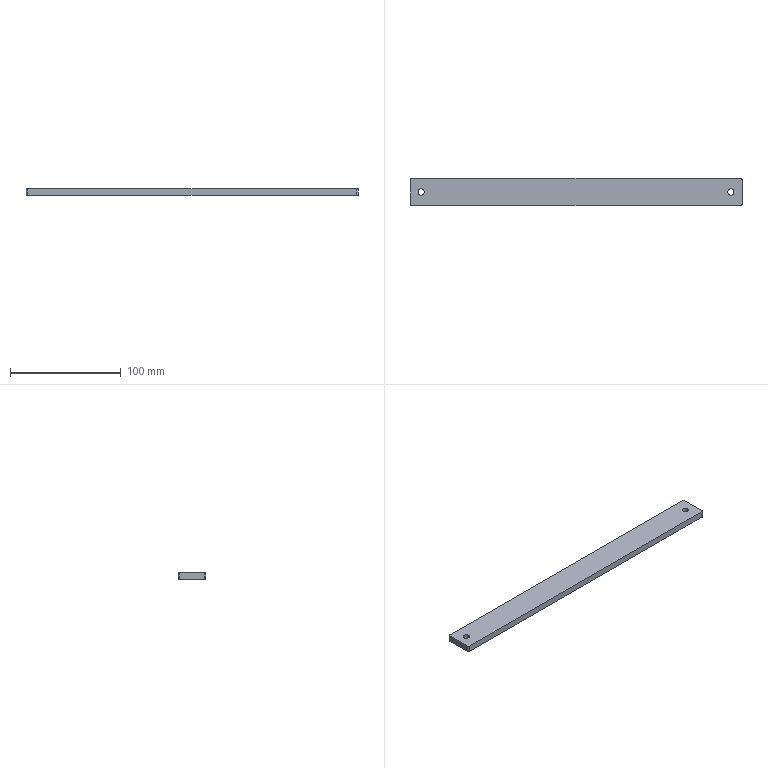Part | STEP file | PN_0032 | 1 solid | 14 faces | box 300 x 25 x 6 mm | volume 44703 mm3 | cylinder 8 | plane 6 | commonest cylinder face diameters 3 x4 5.5 x4
STEP:
#1=CARTESIAN_POINT('',(0.,0.,0.));
#2=DIRECTION('',(0.,0.,1.));
#3=DIRECTION('',(1.,0.,0.));
#4=AXIS2_PLACEMENT_3D('',#1,#2,#3);
#5=CARTESIAN_POINT('',(-137.25,0.,0.));
#6=VERTEX_POINT('',#5);
#7=CARTESIAN_POINT('',(-137.25,0.,6.));
#8=VERTEX_POINT('',#7);
#9=CARTESIAN_POINT('',(-137.25,0.,6.));
#10=DIRECTION('',(0.,0.,1.));
#11=VECTOR('',#10,1.);
#12=LINE('',#9,#11);
#13=CARTESIAN_POINT('',(-140.,0.,6.));
#14=DIRECTION('',(0.,0.,1.));
#15=DIRECTION('',(1.,0.,0.));
#16=AXIS2_PLACEMENT_3D('',#13,#14,#15);
#17=CYLINDRICAL_SURFACE('',#16,2.75);
#18=CARTESIAN_POINT('',(6.283,0.));
#19=DIRECTION('',(0.,1.));
#20=VECTOR('',#19,1.);
#21=LINE('',#18,#20);
#22=(GEOMETRIC_REPRESENTATION_CONTEXT(2)PARAMETRIC_REPRESENTATION_CONTEXT()REPRESENTATION_CONTEXT('',''));
#23=DEFINITIONAL_REPRESENTATION('',(#21),#22);
#24=PCURVE('',#17,#23);
#25=CARTESIAN_POINT('',(-140.,0.,6.));
#26=DIRECTION('',(0.,0.,1.));
#27=DIRECTION('',(1.,0.,0.));
#28=AXIS2_PLACEMENT_3D('',#25,#26,#27);
#29=CYLINDRICAL_SURFACE('',#28,2.75);
#30=CARTESIAN_POINT('',(0.,0.));
#31=DIRECTION('',(0.,1.));
#32=VECTOR('',#31,1.);
#33=LINE('',#30,#32);
#34=(GEOMETRIC_REPRESENTATION_CONTEXT(2)PARAMETRIC_REPRESENTATION_CONTEXT()REPRESENTATION_CONTEXT('',''));
#35=DEFINITIONAL_REPRESENTATION('',(#33),#34);
#36=PCURVE('',#29,#35);
#37=SURFACE_CURVE('',#12,(#24,#36),.PCURVE_S1.);
#38=EDGE_CURVE('',#6,#8,#37,.T.);
#39=ORIENTED_EDGE('',*,*,#38,.T.);
#40=CARTESIAN_POINT('',(-142.75,0.,6.));
#41=VERTEX_POINT('',#40);
#42=CARTESIAN_POINT('',(-140.,0.,6.));
#43=DIRECTION('',(0.,0.,1.));
#44=DIRECTION('',(1.,0.,0.));
#45=AXIS2_PLACEMENT_3D('',#42,#43,#44);
#46=CIRCLE('',#45,2.75);
#47=CARTESIAN_POINT('',(0.,0.));
#48=DIRECTION('',(1.,0.));
#49=VECTOR('',#48,1.);
#50=LINE('',#47,#49);
#51=(GEOMETRIC_REPRESENTATION_CONTEXT(2)PARAMETRIC_REPRESENTATION_CONTEXT()REPRESENTATION_CONTEXT('',''));
#52=DEFINITIONAL_REPRESENTATION('',(#50),#51);
#53=PCURVE('',#17,#52);
#54=CARTESIAN_POINT('',(0.,0.,6.));
#55=DIRECTION('',(0.,0.,1.));
#56=DIRECTION('',(1.,0.,0.));
#57=AXIS2_PLACEMENT_3D('',#54,#55,#56);
#58=PLANE('',#57);
#59=CARTESIAN_POINT('',(-140.,0.));
#60=DIRECTION('',(1.,0.));
#61=AXIS2_PLACEMENT_2D('',#59,#60);
#62=CIRCLE('',#61,2.75);
#63=(GEOMETRIC_REPRESENTATION_CONTEXT(2)PARAMETRIC_REPRESENTATION_CONTEXT()REPRESENTATION_CONTEXT('',''));
#64=DEFINITIONAL_REPRESENTATION('',(#62),#63);
#65=PCURVE('',#58,#64);
#66=SURFACE_CURVE('',#46,(#53,#65),.PCURVE_S1.);
#67=EDGE_CURVE('',#41,#8,#66,.T.);
#68=ORIENTED_EDGE('',*,*,#67,.F.);
#69=CARTESIAN_POINT('',(-142.75,0.,0.));
#70=VERTEX_POINT('',#69);
#71=CARTESIAN_POINT('',(-142.75,0.,6.));
#72=DIRECTION('',(0.,0.,1.));
#73=VECTOR('',#72,1.);
#74=LINE('',#71,#73);
#75=CARTESIAN_POINT('',(3.142,0.));
#76=DIRECTION('',(0.,1.));
#77=VECTOR('',#76,1.);
#78=LINE('',#75,#77);
#79=(GEOMETRIC_REPRESENTATION_CONTEXT(2)PARAMETRIC_REPRESENTATION_CONTEXT()REPRESENTATION_CONTEXT('',''));
#80=DEFINITIONAL_REPRESENTATION('',(#78),#79);
#81=PCURVE('',#17,#80);
#82=CARTESIAN_POINT('',(3.142,0.));
#83=DIRECTION('',(0.,1.));
#84=VECTOR('',#83,1.);
#85=LINE('',#82,#84);
#86=(GEOMETRIC_REPRESENTATION_CONTEXT(2)PARAMETRIC_REPRESENTATION_CONTEXT()REPRESENTATION_CONTEXT('',''));
#87=DEFINITIONAL_REPRESENTATION('',(#85),#86);
#88=PCURVE('',#29,#87);
#89=SURFACE_CURVE('',#74,(#81,#88),.PCURVE_S1.);
#90=EDGE_CURVE('',#70,#41,#89,.T.);
#91=ORIENTED_EDGE('',*,*,#90,.F.);
#92=CARTESIAN_POINT('',(-140.,0.,0.));
#93=DIRECTION('',(0.,0.,1.));
#94=DIRECTION('',(1.,0.,0.));
#95=AXIS2_PLACEMENT_3D('',#92,#93,#94);
#96=CIRCLE('',#95,2.75);
#97=CARTESIAN_POINT('',(0.,-6.));
#98=DIRECTION('',(1.,0.));
#99=VECTOR('',#98,1.);
#100=LINE('',#97,#99);
#101=(GEOMETRIC_REPRESENTATION_CONTEXT(2)PARAMETRIC_REPRESENTATION_CONTEXT()REPRESENTATION_CONTEXT('',''));
#102=DEFINITIONAL_REPRESENTATION('',(#100),#101);
#103=PCURVE('',#17,#102);
#104=CARTESIAN_POINT('',(0.,0.,0.));
#105=DIRECTION('',(0.,0.,1.));
#106=DIRECTION('',(1.,0.,0.));
#107=AXIS2_PLACEMENT_3D('',#104,#105,#106);
#108=PLANE('',#107);
#109=CARTESIAN_POINT('',(-140.,0.));
#110=DIRECTION('',(1.,0.));
#111=AXIS2_PLACEMENT_2D('',#109,#110);
#112=CIRCLE('',#111,2.75);
#113=(GEOMETRIC_REPRESENTATION_CONTEXT(2)PARAMETRIC_REPRESENTATION_CONTEXT()REPRESENTATION_CONTEXT('',''));
#114=DEFINITIONAL_REPRESENTATION('',(#112),#113);
#115=PCURVE('',#108,#114);
#116=SURFACE_CURVE('',#96,(#103,#115),.PCURVE_S1.);
#117=EDGE_CURVE('',#70,#6,#116,.T.);
#118=ORIENTED_EDGE('',*,*,#117,.T.);
#119=EDGE_LOOP('',(#39,#68,#91,#118));
#120=FACE_BOUND('',#119,.F.);
#121=ADVANCED_FACE('',(#120),#17,.F.);
#122=CARTESIAN_POINT('',(142.75,0.,0.));
#123=VERTEX_POINT('',#122);
#124=CARTESIAN_POINT('',(142.75,0.,6.));
#125=VERTEX_POINT('',#124);
#126=CARTESIAN_POINT('',(142.75,0.,6.));
#127=DIRECTION('',(0.,0.,1.));
#128=VECTOR('',#127,1.);
#129=LINE('',#126,#128);
#130=CARTESIAN_POINT('',(140.,0.,6.));
#131=DIRECTION('',(0.,0.,1.));
#132=DIRECTION('',(1.,0.,0.));
#133=AXIS2_PLACEMENT_3D('',#130,#131,#132);
#134=CYLINDRICAL_SURFACE('',#133,2.75);
#135=CARTESIAN_POINT('',(6.283,0.));
#136=DIRECTION('',(0.,1.));
#137=VECTOR('',#136,1.);
#138=LINE('',#135,#137);
#139=(GEOMETRIC_REPRESENTATION_CONTEXT(2)PARAMETRIC_REPRESENTATION_CONTEXT()REPRESENTATION_CONTEXT('',''));
#140=DEFINITIONAL_REPRESENTATION('',(#138),#139);
#141=PCURVE('',#134,#140);
#142=CARTESIAN_POINT('',(140.,0.,6.));
#143=DIRECTION('',(0.,0.,1.));
#144=DIRECTION('',(1.,0.,0.));
#145=AXIS2_PLACEMENT_3D('',#142,#143,#144);
#146=CYLINDRICAL_SURFACE('',#145,2.75);
#147=CARTESIAN_POINT('',(0.,0.));
#148=DIRECTION('',(0.,1.));
#149=VECTOR('',#148,1.);
#150=LINE('',#147,#149);
#151=(GEOMETRIC_REPRESENTATION_CONTEXT(2)PARAMETRIC_REPRESENTATION_CONTEXT()REPRESENTATION_CONTEXT('',''));
#152=DEFINITIONAL_REPRESENTATION('',(#150),#151);
#153=PCURVE('',#146,#152);
#154=SURFACE_CURVE('',#129,(#141,#153),.PCURVE_S1.);
#155=EDGE_CURVE('',#123,#125,#154,.T.);
#156=ORIENTED_EDGE('',*,*,#155,.T.);
#157=CARTESIAN_POINT('',(137.25,0.,6.));
#158=VERTEX_POINT('',#157);
#159=CARTESIAN_POINT('',(140.,0.,6.));
#160=DIRECTION('',(0.,0.,1.));
#161=DIRECTION('',(1.,0.,0.));
#162=AXIS2_PLACEMENT_3D('',#159,#160,#161);
#163=CIRCLE('',#162,2.75);
#164=CARTESIAN_POINT('',(0.,0.));
#165=DIRECTION('',(1.,0.));
#166=VECTOR('',#165,1.);
#167=LINE('',#164,#166);
#168=(GEOMETRIC_REPRESENTATION_CONTEXT(2)PARAMETRIC_REPRESENTATION_CONTEXT()REPRESENTATION_CONTEXT('',''));
#169=DEFINITIONAL_REPRESENTATION('',(#167),#168);
#170=PCURVE('',#134,#169);
#171=CARTESIAN_POINT('',(140.,0.));
#172=DIRECTION('',(1.,0.));
#173=AXIS2_PLACEMENT_2D('',#171,#172);
#174=CIRCLE('',#173,2.75);
#175=(GEOMETRIC_REPRESENTATION_CONTEXT(2)PARAMETRIC_REPRESENTATION_CONTEXT()REPRESENTATION_CONTEXT('',''));
#176=DEFINITIONAL_REPRESENTATION('',(#174),#175);
#177=PCURVE('',#58,#176);
#178=SURFACE_CURVE('',#163,(#170,#177),.PCURVE_S1.);
#179=EDGE_CURVE('',#158,#125,#178,.T.);
#180=ORIENTED_EDGE('',*,*,#179,.F.);
#181=CARTESIAN_POINT('',(137.25,0.,0.));
#182=VERTEX_POINT('',#181);
#183=CARTESIAN_POINT('',(137.25,0.,6.));
#184=DIRECTION('',(0.,0.,1.));
#185=VECTOR('',#184,1.);
#186=LINE('',#183,#185);
#187=CARTESIAN_POINT('',(3.142,0.));
#188=DIRECTION('',(0.,1.));
#189=VECTOR('',#188,1.);
#190=LINE('',#187,#189);
#191=(GEOMETRIC_REPRESENTATION_CONTEXT(2)PARAMETRIC_REPRESENTATION_CONTEXT()REPRESENTATION_CONTEXT('',''));
#192=DEFINITIONAL_REPRESENTATION('',(#190),#191);
#193=PCURVE('',#134,#192);
#194=CARTESIAN_POINT('',(3.142,0.));
#195=DIRECTION('',(0.,1.));
#196=VECTOR('',#195,1.);
#197=LINE('',#194,#196);
#198=(GEOMETRIC_REPRESENTATION_CONTEXT(2)PARAMETRIC_REPRESENTATION_CONTEXT()REPRESENTATION_CONTEXT('',''));
#199=DEFINITIONAL_REPRESENTATION('',(#197),#198);
#200=PCURVE('',#146,#199);
#201=SURFACE_CURVE('',#186,(#193,#200),.PCURVE_S1.);
#202=EDGE_CURVE('',#182,#158,#201,.T.);
#203=ORIENTED_EDGE('',*,*,#202,.F.);
#204=CARTESIAN_POINT('',(140.,0.,0.));
#205=DIRECTION('',(0.,0.,1.));
#206=DIRECTION('',(1.,0.,0.));
#207=AXIS2_PLACEMENT_3D('',#204,#205,#206);
#208=CIRCLE('',#207,2.75);
#209=CARTESIAN_POINT('',(0.,-6.));
#210=DIRECTION('',(1.,0.));
#211=VECTOR('',#210,1.);
#212=LINE('',#209,#211);
#213=(GEOMETRIC_REPRESENTATION_CONTEXT(2)PARAMETRIC_REPRESENTATION_CONTEXT()REPRESENTATION_CONTEXT('',''));
#214=DEFINITIONAL_REPRESENTATION('',(#212),#213);
#215=PCURVE('',#134,#214);
#216=CARTESIAN_POINT('',(140.,0.));
#217=DIRECTION('',(1.,0.));
#218=AXIS2_PLACEMENT_2D('',#216,#217);
#219=CIRCLE('',#218,2.75);
#220=(GEOMETRIC_REPRESENTATION_CONTEXT(2)PARAMETRIC_REPRESENTATION_CONTEXT()REPRESENTATION_CONTEXT('',''));
#221=DEFINITIONAL_REPRESENTATION('',(#219),#220);
#222=PCURVE('',#108,#221);
#223=SURFACE_CURVE('',#208,(#215,#222),.PCURVE_S1.);
#224=EDGE_CURVE('',#182,#123,#223,.T.);
#225=ORIENTED_EDGE('',*,*,#224,.T.);
#226=EDGE_LOOP('',(#156,#180,#203,#225));
#227=FACE_BOUND('',#226,.F.);
#228=ADVANCED_FACE('',(#227),#134,.F.);
#229=CARTESIAN_POINT('',(150.,-11.,6.));
#230=VERTEX_POINT('',#229);
#231=CARTESIAN_POINT('',(150.,11.,6.));
#232=VERTEX_POINT('',#231);
#233=CARTESIAN_POINT('',(150.,12.5,6.));
#234=DIRECTION('',(0.,1.,0.));
#235=VECTOR('',#234,1.);
#236=LINE('',#233,#235);
#237=CARTESIAN_POINT('',(150.,12.5,6.));
#238=DIRECTION('',(-1.,0.,0.));
#239=DIRECTION('',(0.,0.,1.));
#240=AXIS2_PLACEMENT_3D('',#237,#238,#239);
#241=PLANE('',#240);
#242=CARTESIAN_POINT('',(0.,0.));
#243=DIRECTION('',(0.,1.));
#244=VECTOR('',#243,1.);
#245=LINE('',#242,#244);
#246=(GEOMETRIC_REPRESENTATION_CONTEXT(2)PARAMETRIC_REPRESENTATION_CONTEXT()REPRESENTATION_CONTEXT('',''));
#247=DEFINITIONAL_REPRESENTATION('',(#245),#246);
#248=PCURVE('',#241,#247);
#249=CARTESIAN_POINT('',(150.,12.5));
#250=DIRECTION('',(0.,1.));
#251=VECTOR('',#250,1.);
#252=LINE('',#249,#251);
#253=(GEOMETRIC_REPRESENTATION_CONTEXT(2)PARAMETRIC_REPRESENTATION_CONTEXT()REPRESENTATION_CONTEXT('',''));
#254=DEFINITIONAL_REPRESENTATION('',(#252),#253);
#255=PCURVE('',#58,#254);
#256=SURFACE_CURVE('',#236,(#248,#255),.PCURVE_S1.);
#257=EDGE_CURVE('',#230,#232,#256,.T.);
#258=ORIENTED_EDGE('',*,*,#257,.F.);
#259=CARTESIAN_POINT('',(150.,-11.,0.));
#260=VERTEX_POINT('',#259);
#261=CARTESIAN_POINT('',(150.,-11.,6.));
#262=DIRECTION('',(0.,0.,-1.));
#263=VECTOR('',#262,1.);
#264=LINE('',#261,#263);
#265=CARTESIAN_POINT('',(0.,-23.5));
#266=DIRECTION('',(-1.,0.));
#267=VECTOR('',#266,1.);
#268=LINE('',#265,#267);
#269=(GEOMETRIC_REPRESENTATION_CONTEXT(2)PARAMETRIC_REPRESENTATION_CONTEXT()REPRESENTATION_CONTEXT('',''));
#270=DEFINITIONAL_REPRESENTATION('',(#268),#269);
#271=PCURVE('',#241,#270);
#272=CARTESIAN_POINT('',(148.5,-11.,6.));
#273=DIRECTION('',(0.,0.,-1.));
#274=DIRECTION('',(-1.,0.,0.));
#275=AXIS2_PLACEMENT_3D('',#272,#273,#274);
#276=CYLINDRICAL_SURFACE('',#275,1.5);
#277=CARTESIAN_POINT('',(3.142,0.));
#278=DIRECTION('',(0.,1.));
#279=VECTOR('',#278,1.);
#280=LINE('',#277,#279);
#281=(GEOMETRIC_REPRESENTATION_CONTEXT(2)PARAMETRIC_REPRESENTATION_CONTEXT()REPRESENTATION_CONTEXT('',''));
#282=DEFINITIONAL_REPRESENTATION('',(#280),#281);
#283=PCURVE('',#276,#282);
#284=SURFACE_CURVE('',#264,(#271,#283),.PCURVE_S1.);
#285=EDGE_CURVE('',#230,#260,#284,.T.);
#286=ORIENTED_EDGE('',*,*,#285,.T.);
#287=CARTESIAN_POINT('',(150.,11.,0.));
#288=VERTEX_POINT('',#287);
#289=CARTESIAN_POINT('',(150.,12.5,0.));
#290=DIRECTION('',(0.,1.,0.));
#291=VECTOR('',#290,1.);
#292=LINE('',#289,#291);
#293=CARTESIAN_POINT('',(-6.,0.));
#294=DIRECTION('',(0.,1.));
#295=VECTOR('',#294,1.);
#296=LINE('',#293,#295);
#297=(GEOMETRIC_REPRESENTATION_CONTEXT(2)PARAMETRIC_REPRESENTATION_CONTEXT()REPRESENTATION_CONTEXT('',''));
#298=DEFINITIONAL_REPRESENTATION('',(#296),#297);
#299=PCURVE('',#241,#298);
#300=CARTESIAN_POINT('',(150.,12.5));
#301=DIRECTION('',(0.,1.));
#302=VECTOR('',#301,1.);
#303=LINE('',#300,#302);
#304=(GEOMETRIC_REPRESENTATION_CONTEXT(2)PARAMETRIC_REPRESENTATION_CONTEXT()REPRESENTATION_CONTEXT('',''));
#305=DEFINITIONAL_REPRESENTATION('',(#303),#304);
#306=PCURVE('',#108,#305);
#307=SURFACE_CURVE('',#292,(#299,#306),.PCURVE_S1.);
#308=EDGE_CURVE('',#260,#288,#307,.T.);
#309=ORIENTED_EDGE('',*,*,#308,.T.);
#310=CARTESIAN_POINT('',(150.,11.,6.));
#311=DIRECTION('',(0.,0.,1.));
#312=VECTOR('',#311,1.);
#313=LINE('',#310,#312);
#314=CARTESIAN_POINT('',(0.,-1.5));
#315=DIRECTION('',(1.,0.));
#316=VECTOR('',#315,1.);
#317=LINE('',#314,#316);
#318=(GEOMETRIC_REPRESENTATION_CONTEXT(2)PARAMETRIC_REPRESENTATION_CONTEXT()REPRESENTATION_CONTEXT('',''));
#319=DEFINITIONAL_REPRESENTATION('',(#317),#318);
#320=PCURVE('',#241,#319);
#321=CARTESIAN_POINT('',(148.5,11.,6.));
#322=DIRECTION('',(0.,0.,-1.));
#323=DIRECTION('',(-1.,0.,0.));
#324=AXIS2_PLACEMENT_3D('',#321,#322,#323);
#325=CYLINDRICAL_SURFACE('',#324,1.5);
#326=CARTESIAN_POINT('',(3.142,0.));
#327=DIRECTION('',(0.,-1.));
#328=VECTOR('',#327,1.);
#329=LINE('',#326,#328);
#330=(GEOMETRIC_REPRESENTATION_CONTEXT(2)PARAMETRIC_REPRESENTATION_CONTEXT()REPRESENTATION_CONTEXT('',''));
#331=DEFINITIONAL_REPRESENTATION('',(#329),#330);
#332=PCURVE('',#325,#331);
#333=SURFACE_CURVE('',#313,(#320,#332),.PCURVE_S1.);
#334=EDGE_CURVE('',#288,#232,#333,.T.);
#335=ORIENTED_EDGE('',*,*,#334,.T.);
#336=EDGE_LOOP('',(#258,#286,#309,#335));
#337=FACE_BOUND('',#336,.T.);
#338=ADVANCED_FACE('',(#337),#241,.F.);
#339=CARTESIAN_POINT('',(148.5,12.5,6.));
#340=VERTEX_POINT('',#339);
#341=CARTESIAN_POINT('',(-148.5,12.5,6.));
#342=VERTEX_POINT('',#341);
#343=CARTESIAN_POINT('',(-150.,12.5,6.));
#344=DIRECTION('',(-1.,0.,0.));
#345=VECTOR('',#344,1.);
#346=LINE('',#343,#345);
#347=CARTESIAN_POINT('',(-150.,12.5,6.));
#348=DIRECTION('',(0.,-1.,0.));
#349=DIRECTION('',(0.,0.,-1.));
#350=AXIS2_PLACEMENT_3D('',#347,#348,#349);
#351=PLANE('',#350);
#352=CARTESIAN_POINT('',(0.,0.));
#353=DIRECTION('',(0.,-1.));
#354=VECTOR('',#353,1.);
#355=LINE('',#352,#354);
#356=(GEOMETRIC_REPRESENTATION_CONTEXT(2)PARAMETRIC_REPRESENTATION_CONTEXT()REPRESENTATION_CONTEXT('',''));
#357=DEFINITIONAL_REPRESENTATION('',(#355),#356);
#358=PCURVE('',#351,#357);
#359=CARTESIAN_POINT('',(-150.,12.5));
#360=DIRECTION('',(-1.,0.));
#361=VECTOR('',#360,1.);
#362=LINE('',#359,#361);
#363=(GEOMETRIC_REPRESENTATION_CONTEXT(2)PARAMETRIC_REPRESENTATION_CONTEXT()REPRESENTATION_CONTEXT('',''));
#364=DEFINITIONAL_REPRESENTATION('',(#362),#363);
#365=PCURVE('',#58,#364);
#366=SURFACE_CURVE('',#346,(#358,#365),.PCURVE_S1.);
#367=EDGE_CURVE('',#340,#342,#366,.T.);
#368=ORIENTED_EDGE('',*,*,#367,.F.);
#369=CARTESIAN_POINT('',(148.5,12.5,0.));
#370=VERTEX_POINT('',#369);
#371=CARTESIAN_POINT('',(148.5,12.5,6.));
#372=DIRECTION('',(0.,0.,-1.));
#373=VECTOR('',#372,1.);
#374=LINE('',#371,#373);
#375=CARTESIAN_POINT('',(0.,298.5));
#376=DIRECTION('',(1.,0.));
#377=VECTOR('',#376,1.);
#378=LINE('',#375,#377);
#379=(GEOMETRIC_REPRESENTATION_CONTEXT(2)PARAMETRIC_REPRESENTATION_CONTEXT()REPRESENTATION_CONTEXT('',''));
#380=DEFINITIONAL_REPRESENTATION('',(#378),#379);
#381=PCURVE('',#351,#380);
#382=CARTESIAN_POINT('',(1.571,0.));
#383=DIRECTION('',(0.,1.));
#384=VECTOR('',#383,1.);
#385=LINE('',#382,#384);
#386=(GEOMETRIC_REPRESENTATION_CONTEXT(2)PARAMETRIC_REPRESENTATION_CONTEXT()REPRESENTATION_CONTEXT('',''));
#387=DEFINITIONAL_REPRESENTATION('',(#385),#386);
#388=PCURVE('',#325,#387);
#389=SURFACE_CURVE('',#374,(#381,#388),.PCURVE_S1.);
#390=EDGE_CURVE('',#340,#370,#389,.T.);
#391=ORIENTED_EDGE('',*,*,#390,.T.);
#392=CARTESIAN_POINT('',(-148.5,12.5,0.));
#393=VERTEX_POINT('',#392);
#394=CARTESIAN_POINT('',(-150.,12.5,0.));
#395=DIRECTION('',(-1.,0.,0.));
#396=VECTOR('',#395,1.);
#397=LINE('',#394,#396);
#398=CARTESIAN_POINT('',(6.,0.));
#399=DIRECTION('',(0.,-1.));
#400=VECTOR('',#399,1.);
#401=LINE('',#398,#400);
#402=(GEOMETRIC_REPRESENTATION_CONTEXT(2)PARAMETRIC_REPRESENTATION_CONTEXT()REPRESENTATION_CONTEXT('',''));
#403=DEFINITIONAL_REPRESENTATION('',(#401),#402);
#404=PCURVE('',#351,#403);
#405=CARTESIAN_POINT('',(-150.,12.5));
#406=DIRECTION('',(-1.,0.));
#407=VECTOR('',#406,1.);
#408=LINE('',#405,#407);
#409=(GEOMETRIC_REPRESENTATION_CONTEXT(2)PARAMETRIC_REPRESENTATION_CONTEXT()REPRESENTATION_CONTEXT('',''));
#410=DEFINITIONAL_REPRESENTATION('',(#408),#409);
#411=PCURVE('',#108,#410);
#412=SURFACE_CURVE('',#397,(#404,#411),.PCURVE_S1.);
#413=EDGE_CURVE('',#370,#393,#412,.T.);
#414=ORIENTED_EDGE('',*,*,#413,.T.);
#415=CARTESIAN_POINT('',(-148.5,12.5,6.));
#416=DIRECTION('',(0.,0.,1.));
#417=VECTOR('',#416,1.);
#418=LINE('',#415,#417);
#419=CARTESIAN_POINT('',(0.,1.5));
#420=DIRECTION('',(-1.,0.));
#421=VECTOR('',#420,1.);
#422=LINE('',#419,#421);
#423=(GEOMETRIC_REPRESENTATION_CONTEXT(2)PARAMETRIC_REPRESENTATION_CONTEXT()REPRESENTATION_CONTEXT('',''));
#424=DEFINITIONAL_REPRESENTATION('',(#422),#423);
#425=PCURVE('',#351,#424);
#426=CARTESIAN_POINT('',(-148.5,11.,6.));
#427=DIRECTION('',(0.,0.,-1.));
#428=DIRECTION('',(-1.,0.,0.));
#429=AXIS2_PLACEMENT_3D('',#426,#427,#428);
#430=CYLINDRICAL_SURFACE('',#429,1.5);
#431=CARTESIAN_POINT('',(1.571,0.));
#432=DIRECTION('',(0.,-1.));
#433=VECTOR('',#432,1.);
#434=LINE('',#431,#433);
#435=(GEOMETRIC_REPRESENTATION_CONTEXT(2)PARAMETRIC_REPRESENTATION_CONTEXT()REPRESENTATION_CONTEXT('',''));
#436=DEFINITIONAL_REPRESENTATION('',(#434),#435);
#437=PCURVE('',#430,#436);
#438=SURFACE_CURVE('',#418,(#425,#437),.PCURVE_S1.);
#439=EDGE_CURVE('',#393,#342,#438,.T.);
#440=ORIENTED_EDGE('',*,*,#439,.T.);
#441=EDGE_LOOP('',(#368,#391,#414,#440));
#442=FACE_BOUND('',#441,.T.);
#443=ADVANCED_FACE('',(#442),#351,.F.);
#444=CARTESIAN_POINT('',(-150.,11.,0.));
#445=VERTEX_POINT('',#444);
#446=CARTESIAN_POINT('',(-150.,-11.,0.));
#447=VERTEX_POINT('',#446);
#448=CARTESIAN_POINT('',(-150.,12.5,0.));
#449=DIRECTION('',(0.,-1.,0.));
#450=VECTOR('',#449,1.);
#451=LINE('',#448,#450);
#452=CARTESIAN_POINT('',(-150.,12.5,6.));
#453=DIRECTION('',(1.,0.,0.));
#454=DIRECTION('',(0.,0.,-1.));
#455=AXIS2_PLACEMENT_3D('',#452,#453,#454);
#456=PLANE('',#455);
#457=CARTESIAN_POINT('',(6.,0.));
#458=DIRECTION('',(0.,-1.));
#459=VECTOR('',#458,1.);
#460=LINE('',#457,#459);
#461=(GEOMETRIC_REPRESENTATION_CONTEXT(2)PARAMETRIC_REPRESENTATION_CONTEXT()REPRESENTATION_CONTEXT('',''));
#462=DEFINITIONAL_REPRESENTATION('',(#460),#461);
#463=PCURVE('',#456,#462);
#464=CARTESIAN_POINT('',(-150.,12.5));
#465=DIRECTION('',(0.,-1.));
#466=VECTOR('',#465,1.);
#467=LINE('',#464,#466);
#468=(GEOMETRIC_REPRESENTATION_CONTEXT(2)PARAMETRIC_REPRESENTATION_CONTEXT()REPRESENTATION_CONTEXT('',''));
#469=DEFINITIONAL_REPRESENTATION('',(#467),#468);
#470=PCURVE('',#108,#469);
#471=SURFACE_CURVE('',#451,(#463,#470),.PCURVE_S1.);
#472=EDGE_CURVE('',#445,#447,#471,.T.);
#473=ORIENTED_EDGE('',*,*,#472,.T.);
#474=CARTESIAN_POINT('',(-150.,-11.,6.));
#475=VERTEX_POINT('',#474);
#476=CARTESIAN_POINT('',(-150.,-11.,6.));
#477=DIRECTION('',(0.,0.,1.));
#478=VECTOR('',#477,1.);
#479=LINE('',#476,#478);
#480=CARTESIAN_POINT('',(0.,-23.5));
#481=DIRECTION('',(-1.,0.));
#482=VECTOR('',#481,1.);
#483=LINE('',#480,#482);
#484=(GEOMETRIC_REPRESENTATION_CONTEXT(2)PARAMETRIC_REPRESENTATION_CONTEXT()REPRESENTATION_CONTEXT('',''));
#485=DEFINITIONAL_REPRESENTATION('',(#483),#484);
#486=PCURVE('',#456,#485);
#487=CARTESIAN_POINT('',(-148.5,-11.,6.));
#488=DIRECTION('',(0.,0.,-1.));
#489=DIRECTION('',(-1.,0.,0.));
#490=AXIS2_PLACEMENT_3D('',#487,#488,#489);
#491=CYLINDRICAL_SURFACE('',#490,1.5);
#492=CARTESIAN_POINT('',(6.283,0.));
#493=DIRECTION('',(0.,-1.));
#494=VECTOR('',#493,1.);
#495=LINE('',#492,#494);
#496=(GEOMETRIC_REPRESENTATION_CONTEXT(2)PARAMETRIC_REPRESENTATION_CONTEXT()REPRESENTATION_CONTEXT('',''));
#497=DEFINITIONAL_REPRESENTATION('',(#495),#496);
#498=PCURVE('',#491,#497);
#499=SURFACE_CURVE('',#479,(#486,#498),.PCURVE_S1.);
#500=EDGE_CURVE('',#447,#475,#499,.T.);
#501=ORIENTED_EDGE('',*,*,#500,.T.);
#502=CARTESIAN_POINT('',(-150.,11.,6.));
#503=VERTEX_POINT('',#502);
#504=CARTESIAN_POINT('',(-150.,12.5,6.));
#505=DIRECTION('',(0.,-1.,0.));
#506=VECTOR('',#505,1.);
#507=LINE('',#504,#506);
#508=CARTESIAN_POINT('',(0.,0.));
#509=DIRECTION('',(0.,-1.));
#510=VECTOR('',#509,1.);
#511=LINE('',#508,#510);
#512=(GEOMETRIC_REPRESENTATION_CONTEXT(2)PARAMETRIC_REPRESENTATION_CONTEXT()REPRESENTATION_CONTEXT('',''));
#513=DEFINITIONAL_REPRESENTATION('',(#511),#512);
#514=PCURVE('',#456,#513);
#515=CARTESIAN_POINT('',(-150.,12.5));
#516=DIRECTION('',(0.,-1.));
#517=VECTOR('',#516,1.);
#518=LINE('',#515,#517);
#519=(GEOMETRIC_REPRESENTATION_CONTEXT(2)PARAMETRIC_REPRESENTATION_CONTEXT()REPRESENTATION_CONTEXT('',''));
#520=DEFINITIONAL_REPRESENTATION('',(#518),#519);
#521=PCURVE('',#58,#520);
#522=SURFACE_CURVE('',#507,(#514,#521),.PCURVE_S1.);
#523=EDGE_CURVE('',#503,#475,#522,.T.);
#524=ORIENTED_EDGE('',*,*,#523,.F.);
#525=CARTESIAN_POINT('',(-150.,11.,6.));
#526=DIRECTION('',(0.,0.,-1.));
#527=VECTOR('',#526,1.);
#528=LINE('',#525,#527);
#529=CARTESIAN_POINT('',(0.,-1.5));
#530=DIRECTION('',(1.,0.));
#531=VECTOR('',#530,1.);
#532=LINE('',#529,#531);
#533=(GEOMETRIC_REPRESENTATION_CONTEXT(2)PARAMETRIC_REPRESENTATION_CONTEXT()REPRESENTATION_CONTEXT('',''));
#534=DEFINITIONAL_REPRESENTATION('',(#532),#533);
#535=PCURVE('',#456,#534);
#536=CARTESIAN_POINT('',(0.,0.));
#537=DIRECTION('',(0.,1.));
#538=VECTOR('',#537,1.);
#539=LINE('',#536,#538);
#540=(GEOMETRIC_REPRESENTATION_CONTEXT(2)PARAMETRIC_REPRESENTATION_CONTEXT()REPRESENTATION_CONTEXT('',''));
#541=DEFINITIONAL_REPRESENTATION('',(#539),#540);
#542=PCURVE('',#430,#541);
#543=SURFACE_CURVE('',#528,(#535,#542),.PCURVE_S1.);
#544=EDGE_CURVE('',#503,#445,#543,.T.);
#545=ORIENTED_EDGE('',*,*,#544,.T.);
#546=EDGE_LOOP('',(#473,#501,#524,#545));
#547=FACE_BOUND('',#546,.T.);
#548=ADVANCED_FACE('',(#547),#456,.F.);
#549=CARTESIAN_POINT('',(-148.5,-12.5,0.));
#550=VERTEX_POINT('',#549);
#551=CARTESIAN_POINT('',(148.5,-12.5,0.));
#552=VERTEX_POINT('',#551);
#553=CARTESIAN_POINT('',(-150.,-12.5,0.));
#554=DIRECTION('',(1.,0.,0.));
#555=VECTOR('',#554,1.);
#556=LINE('',#553,#555);
#557=CARTESIAN_POINT('',(-150.,-12.5,6.));
#558=DIRECTION('',(0.,1.,0.));
#559=DIRECTION('',(0.,0.,1.));
#560=AXIS2_PLACEMENT_3D('',#557,#558,#559);
#561=PLANE('',#560);
#562=CARTESIAN_POINT('',(-6.,0.));
#563=DIRECTION('',(0.,1.));
#564=VECTOR('',#563,1.);
#565=LINE('',#562,#564);
#566=(GEOMETRIC_REPRESENTATION_CONTEXT(2)PARAMETRIC_REPRESENTATION_CONTEXT()REPRESENTATION_CONTEXT('',''));
#567=DEFINITIONAL_REPRESENTATION('',(#565),#566);
#568=PCURVE('',#561,#567);
#569=CARTESIAN_POINT('',(-150.,-12.5));
#570=DIRECTION('',(1.,0.));
#571=VECTOR('',#570,1.);
#572=LINE('',#569,#571);
#573=(GEOMETRIC_REPRESENTATION_CONTEXT(2)PARAMETRIC_REPRESENTATION_CONTEXT()REPRESENTATION_CONTEXT('',''));
#574=DEFINITIONAL_REPRESENTATION('',(#572),#573);
#575=PCURVE('',#108,#574);
#576=SURFACE_CURVE('',#556,(#568,#575),.PCURVE_S1.);
#577=EDGE_CURVE('',#550,#552,#576,.T.);
#578=ORIENTED_EDGE('',*,*,#577,.T.);
#579=CARTESIAN_POINT('',(148.5,-12.5,6.));
#580=VERTEX_POINT('',#579);
#581=CARTESIAN_POINT('',(148.5,-12.5,6.));
#582=DIRECTION('',(0.,0.,1.));
#583=VECTOR('',#582,1.);
#584=LINE('',#581,#583);
#585=CARTESIAN_POINT('',(0.,298.5));
#586=DIRECTION('',(1.,0.));
#587=VECTOR('',#586,1.);
#588=LINE('',#585,#587);
#589=(GEOMETRIC_REPRESENTATION_CONTEXT(2)PARAMETRIC_REPRESENTATION_CONTEXT()REPRESENTATION_CONTEXT('',''));
#590=DEFINITIONAL_REPRESENTATION('',(#588),#589);
#591=PCURVE('',#561,#590);
#592=CARTESIAN_POINT('',(4.712,0.));
#593=DIRECTION('',(0.,-1.));
#594=VECTOR('',#593,1.);
#595=LINE('',#592,#594);
#596=(GEOMETRIC_REPRESENTATION_CONTEXT(2)PARAMETRIC_REPRESENTATION_CONTEXT()REPRESENTATION_CONTEXT('',''));
#597=DEFINITIONAL_REPRESENTATION('',(#595),#596);
#598=PCURVE('',#276,#597);
#599=SURFACE_CURVE('',#584,(#591,#598),.PCURVE_S1.);
#600=EDGE_CURVE('',#552,#580,#599,.T.);
#601=ORIENTED_EDGE('',*,*,#600,.T.);
#602=CARTESIAN_POINT('',(-148.5,-12.5,6.));
#603=VERTEX_POINT('',#602);
#604=CARTESIAN_POINT('',(-150.,-12.5,6.));
#605=DIRECTION('',(1.,0.,0.));
#606=VECTOR('',#605,1.);
#607=LINE('',#604,#606);
#608=CARTESIAN_POINT('',(0.,0.));
#609=DIRECTION('',(0.,1.));
#610=VECTOR('',#609,1.);
#611=LINE('',#608,#610);
#612=(GEOMETRIC_REPRESENTATION_CONTEXT(2)PARAMETRIC_REPRESENTATION_CONTEXT()REPRESENTATION_CONTEXT('',''));
#613=DEFINITIONAL_REPRESENTATION('',(#611),#612);
#614=PCURVE('',#561,#613);
#615=CARTESIAN_POINT('',(-150.,-12.5));
#616=DIRECTION('',(1.,0.));
#617=VECTOR('',#616,1.);
#618=LINE('',#615,#617);
#619=(GEOMETRIC_REPRESENTATION_CONTEXT(2)PARAMETRIC_REPRESENTATION_CONTEXT()REPRESENTATION_CONTEXT('',''));
#620=DEFINITIONAL_REPRESENTATION('',(#618),#619);
#621=PCURVE('',#58,#620);
#622=SURFACE_CURVE('',#607,(#614,#621),.PCURVE_S1.);
#623=EDGE_CURVE('',#603,#580,#622,.T.);
#624=ORIENTED_EDGE('',*,*,#623,.F.);
#625=CARTESIAN_POINT('',(-148.5,-12.5,6.));
#626=DIRECTION('',(0.,0.,-1.));
#627=VECTOR('',#626,1.);
#628=LINE('',#625,#627);
#629=CARTESIAN_POINT('',(0.,1.5));
#630=DIRECTION('',(-1.,0.));
#631=VECTOR('',#630,1.);
#632=LINE('',#629,#631);
#633=(GEOMETRIC_REPRESENTATION_CONTEXT(2)PARAMETRIC_REPRESENTATION_CONTEXT()REPRESENTATION_CONTEXT('',''));
#634=DEFINITIONAL_REPRESENTATION('',(#632),#633);
#635=PCURVE('',#561,#634);
#636=CARTESIAN_POINT('',(4.712,0.));
#637=DIRECTION('',(0.,1.));
#638=VECTOR('',#637,1.);
#639=LINE('',#636,#638);
#640=(GEOMETRIC_REPRESENTATION_CONTEXT(2)PARAMETRIC_REPRESENTATION_CONTEXT()REPRESENTATION_CONTEXT('',''));
#641=DEFINITIONAL_REPRESENTATION('',(#639),#640);
#642=PCURVE('',#491,#641);
#643=SURFACE_CURVE('',#628,(#635,#642),.PCURVE_S1.);
#644=EDGE_CURVE('',#603,#550,#643,.T.);
#645=ORIENTED_EDGE('',*,*,#644,.T.);
#646=EDGE_LOOP('',(#578,#601,#624,#645));
#647=FACE_BOUND('',#646,.T.);
#648=ADVANCED_FACE('',(#647),#561,.F.);
#649=CARTESIAN_POINT('',(-140.,0.,6.));
#650=DIRECTION('',(0.,0.,1.));
#651=DIRECTION('',(1.,0.,0.));
#652=AXIS2_PLACEMENT_3D('',#649,#650,#651);
#653=CIRCLE('',#652,2.75);
#654=CARTESIAN_POINT('',(-140.,0.));
#655=DIRECTION('',(1.,0.));
#656=AXIS2_PLACEMENT_2D('',#654,#655);
#657=CIRCLE('',#656,2.75);
#658=(GEOMETRIC_REPRESENTATION_CONTEXT(2)PARAMETRIC_REPRESENTATION_CONTEXT()REPRESENTATION_CONTEXT('',''));
#659=DEFINITIONAL_REPRESENTATION('',(#657),#658);
#660=PCURVE('',#58,#659);
#661=CARTESIAN_POINT('',(0.,0.));
#662=DIRECTION('',(1.,0.));
#663=VECTOR('',#662,1.);
#664=LINE('',#661,#663);
#665=(GEOMETRIC_REPRESENTATION_CONTEXT(2)PARAMETRIC_REPRESENTATION_CONTEXT()REPRESENTATION_CONTEXT('',''));
#666=DEFINITIONAL_REPRESENTATION('',(#664),#665);
#667=PCURVE('',#29,#666);
#668=SURFACE_CURVE('',#653,(#660,#667),.PCURVE_S1.);
#669=EDGE_CURVE('',#8,#41,#668,.T.);
#670=ORIENTED_EDGE('',*,*,#669,.F.);
#671=ORIENTED_EDGE('',*,*,#67,.F.);
#672=EDGE_LOOP('',(#670,#671));
#673=FACE_BOUND('',#672,.T.);
#674=CARTESIAN_POINT('',(140.,0.,6.));
#675=DIRECTION('',(0.,0.,1.));
#676=DIRECTION('',(1.,0.,0.));
#677=AXIS2_PLACEMENT_3D('',#674,#675,#676);
#678=CIRCLE('',#677,2.75);
#679=CARTESIAN_POINT('',(140.,0.));
#680=DIRECTION('',(1.,0.));
#681=AXIS2_PLACEMENT_2D('',#679,#680);
#682=CIRCLE('',#681,2.75);
#683=(GEOMETRIC_REPRESENTATION_CONTEXT(2)PARAMETRIC_REPRESENTATION_CONTEXT()REPRESENTATION_CONTEXT('',''));
#684=DEFINITIONAL_REPRESENTATION('',(#682),#683);
#685=PCURVE('',#58,#684);
#686=CARTESIAN_POINT('',(0.,0.));
#687=DIRECTION('',(1.,0.));
#688=VECTOR('',#687,1.);
#689=LINE('',#686,#688);
#690=(GEOMETRIC_REPRESENTATION_CONTEXT(2)PARAMETRIC_REPRESENTATION_CONTEXT()REPRESENTATION_CONTEXT('',''));
#691=DEFINITIONAL_REPRESENTATION('',(#689),#690);
#692=PCURVE('',#146,#691);
#693=SURFACE_CURVE('',#678,(#685,#692),.PCURVE_S1.);
#694=EDGE_CURVE('',#125,#158,#693,.T.);
#695=ORIENTED_EDGE('',*,*,#694,.F.);
#696=ORIENTED_EDGE('',*,*,#179,.F.);
#697=EDGE_LOOP('',(#695,#696));
#698=FACE_BOUND('',#697,.T.);
#699=ORIENTED_EDGE('',*,*,#623,.T.);
#700=CARTESIAN_POINT('',(148.5,-11.,6.));
#701=DIRECTION('',(0.,0.,1.));
#702=DIRECTION('',(1.,0.,0.));
#703=AXIS2_PLACEMENT_3D('',#700,#701,#702);
#704=CIRCLE('',#703,1.5);
#705=CARTESIAN_POINT('',(148.5,-11.));
#706=DIRECTION('',(1.,0.));
#707=AXIS2_PLACEMENT_2D('',#705,#706);
#708=CIRCLE('',#707,1.5);
#709=(GEOMETRIC_REPRESENTATION_CONTEXT(2)PARAMETRIC_REPRESENTATION_CONTEXT()REPRESENTATION_CONTEXT('',''));
#710=DEFINITIONAL_REPRESENTATION('',(#708),#709);
#711=PCURVE('',#58,#710);
#712=CARTESIAN_POINT('',(9.425,0.));
#713=DIRECTION('',(-1.,0.));
#714=VECTOR('',#713,1.);
#715=LINE('',#712,#714);
#716=(GEOMETRIC_REPRESENTATION_CONTEXT(2)PARAMETRIC_REPRESENTATION_CONTEXT()REPRESENTATION_CONTEXT('',''));
#717=DEFINITIONAL_REPRESENTATION('',(#715),#716);
#718=PCURVE('',#276,#717);
#719=SURFACE_CURVE('',#704,(#711,#718),.PCURVE_S1.);
#720=EDGE_CURVE('',#580,#230,#719,.T.);
#721=ORIENTED_EDGE('',*,*,#720,.T.);
#722=ORIENTED_EDGE('',*,*,#257,.T.);
#723=CARTESIAN_POINT('',(148.5,11.,6.));
#724=DIRECTION('',(0.,0.,1.));
#725=DIRECTION('',(1.,0.,0.));
#726=AXIS2_PLACEMENT_3D('',#723,#724,#725);
#727=CIRCLE('',#726,1.5);
#728=CARTESIAN_POINT('',(148.5,11.));
#729=DIRECTION('',(1.,0.));
#730=AXIS2_PLACEMENT_2D('',#728,#729);
#731=CIRCLE('',#730,1.5);
#732=(GEOMETRIC_REPRESENTATION_CONTEXT(2)PARAMETRIC_REPRESENTATION_CONTEXT()REPRESENTATION_CONTEXT('',''));
#733=DEFINITIONAL_REPRESENTATION('',(#731),#732);
#734=PCURVE('',#58,#733);
#735=CARTESIAN_POINT('',(3.142,0.));
#736=DIRECTION('',(-1.,0.));
#737=VECTOR('',#736,1.);
#738=LINE('',#735,#737);
#739=(GEOMETRIC_REPRESENTATION_CONTEXT(2)PARAMETRIC_REPRESENTATION_CONTEXT()REPRESENTATION_CONTEXT('',''));
#740=DEFINITIONAL_REPRESENTATION('',(#738),#739);
#741=PCURVE('',#325,#740);
#742=SURFACE_CURVE('',#727,(#734,#741),.PCURVE_S1.);
#743=EDGE_CURVE('',#232,#340,#742,.T.);
#744=ORIENTED_EDGE('',*,*,#743,.T.);
#745=ORIENTED_EDGE('',*,*,#367,.T.);
#746=CARTESIAN_POINT('',(-148.5,11.,6.));
#747=DIRECTION('',(0.,0.,1.));
#748=DIRECTION('',(1.,0.,0.));
#749=AXIS2_PLACEMENT_3D('',#746,#747,#748);
#750=CIRCLE('',#749,1.5);
#751=CARTESIAN_POINT('',(-148.5,11.));
#752=DIRECTION('',(1.,0.));
#753=AXIS2_PLACEMENT_2D('',#751,#752);
#754=CIRCLE('',#753,1.5);
#755=(GEOMETRIC_REPRESENTATION_CONTEXT(2)PARAMETRIC_REPRESENTATION_CONTEXT()REPRESENTATION_CONTEXT('',''));
#756=DEFINITIONAL_REPRESENTATION('',(#754),#755);
#757=PCURVE('',#58,#756);
#758=CARTESIAN_POINT('',(3.142,0.));
#759=DIRECTION('',(-1.,0.));
#760=VECTOR('',#759,1.);
#761=LINE('',#758,#760);
#762=(GEOMETRIC_REPRESENTATION_CONTEXT(2)PARAMETRIC_REPRESENTATION_CONTEXT()REPRESENTATION_CONTEXT('',''));
#763=DEFINITIONAL_REPRESENTATION('',(#761),#762);
#764=PCURVE('',#430,#763);
#765=SURFACE_CURVE('',#750,(#757,#764),.PCURVE_S1.);
#766=EDGE_CURVE('',#342,#503,#765,.T.);
#767=ORIENTED_EDGE('',*,*,#766,.T.);
#768=ORIENTED_EDGE('',*,*,#523,.T.);
#769=CARTESIAN_POINT('',(-148.5,-11.,6.));
#770=DIRECTION('',(0.,0.,1.));
#771=DIRECTION('',(1.,0.,0.));
#772=AXIS2_PLACEMENT_3D('',#769,#770,#771);
#773=CIRCLE('',#772,1.5);
#774=CARTESIAN_POINT('',(-148.5,-11.));
#775=DIRECTION('',(1.,0.));
#776=AXIS2_PLACEMENT_2D('',#774,#775);
#777=CIRCLE('',#776,1.5);
#778=(GEOMETRIC_REPRESENTATION_CONTEXT(2)PARAMETRIC_REPRESENTATION_CONTEXT()REPRESENTATION_CONTEXT('',''));
#779=DEFINITIONAL_REPRESENTATION('',(#777),#778);
#780=PCURVE('',#58,#779);
#781=CARTESIAN_POINT('',(9.425,0.));
#782=DIRECTION('',(-1.,0.));
#783=VECTOR('',#782,1.);
#784=LINE('',#781,#783);
#785=(GEOMETRIC_REPRESENTATION_CONTEXT(2)PARAMETRIC_REPRESENTATION_CONTEXT()REPRESENTATION_CONTEXT('',''));
#786=DEFINITIONAL_REPRESENTATION('',(#784),#785);
#787=PCURVE('',#491,#786);
#788=SURFACE_CURVE('',#773,(#780,#787),.PCURVE_S1.);
#789=EDGE_CURVE('',#475,#603,#788,.T.);
#790=ORIENTED_EDGE('',*,*,#789,.T.);
#791=EDGE_LOOP('',(#699,#721,#722,#744,#745,#767,#768,#790));
#792=FACE_BOUND('',#791,.T.);
#793=ADVANCED_FACE('',(#673,#698,#792),#58,.T.);
#794=CARTESIAN_POINT('',(-140.,0.,0.));
#795=DIRECTION('',(0.,0.,1.));
#796=DIRECTION('',(1.,0.,0.));
#797=AXIS2_PLACEMENT_3D('',#794,#795,#796);
#798=CIRCLE('',#797,2.75);
#799=CARTESIAN_POINT('',(-140.,0.));
#800=DIRECTION('',(1.,0.));
#801=AXIS2_PLACEMENT_2D('',#799,#800);
#802=CIRCLE('',#801,2.75);
#803=(GEOMETRIC_REPRESENTATION_CONTEXT(2)PARAMETRIC_REPRESENTATION_CONTEXT()REPRESENTATION_CONTEXT('',''));
#804=DEFINITIONAL_REPRESENTATION('',(#802),#803);
#805=PCURVE('',#108,#804);
#806=CARTESIAN_POINT('',(0.,-6.));
#807=DIRECTION('',(1.,0.));
#808=VECTOR('',#807,1.);
#809=LINE('',#806,#808);
#810=(GEOMETRIC_REPRESENTATION_CONTEXT(2)PARAMETRIC_REPRESENTATION_CONTEXT()REPRESENTATION_CONTEXT('',''));
#811=DEFINITIONAL_REPRESENTATION('',(#809),#810);
#812=PCURVE('',#29,#811);
#813=SURFACE_CURVE('',#798,(#805,#812),.PCURVE_S1.);
#814=EDGE_CURVE('',#6,#70,#813,.T.);
#815=ORIENTED_EDGE('',*,*,#814,.T.);
#816=ORIENTED_EDGE('',*,*,#117,.T.);
#817=EDGE_LOOP('',(#815,#816));
#818=FACE_BOUND('',#817,.T.);
#819=CARTESIAN_POINT('',(140.,0.,0.));
#820=DIRECTION('',(0.,0.,1.));
#821=DIRECTION('',(1.,0.,0.));
#822=AXIS2_PLACEMENT_3D('',#819,#820,#821);
#823=CIRCLE('',#822,2.75);
#824=CARTESIAN_POINT('',(140.,0.));
#825=DIRECTION('',(1.,0.));
#826=AXIS2_PLACEMENT_2D('',#824,#825);
#827=CIRCLE('',#826,2.75);
#828=(GEOMETRIC_REPRESENTATION_CONTEXT(2)PARAMETRIC_REPRESENTATION_CONTEXT()REPRESENTATION_CONTEXT('',''));
#829=DEFINITIONAL_REPRESENTATION('',(#827),#828);
#830=PCURVE('',#108,#829);
#831=CARTESIAN_POINT('',(0.,-6.));
#832=DIRECTION('',(1.,0.));
#833=VECTOR('',#832,1.);
#834=LINE('',#831,#833);
#835=(GEOMETRIC_REPRESENTATION_CONTEXT(2)PARAMETRIC_REPRESENTATION_CONTEXT()REPRESENTATION_CONTEXT('',''));
#836=DEFINITIONAL_REPRESENTATION('',(#834),#835);
#837=PCURVE('',#146,#836);
#838=SURFACE_CURVE('',#823,(#830,#837),.PCURVE_S1.);
#839=EDGE_CURVE('',#123,#182,#838,.T.);
#840=ORIENTED_EDGE('',*,*,#839,.T.);
#841=ORIENTED_EDGE('',*,*,#224,.T.);
#842=EDGE_LOOP('',(#840,#841));
#843=FACE_BOUND('',#842,.T.);
#844=ORIENTED_EDGE('',*,*,#308,.F.);
#845=CARTESIAN_POINT('',(148.5,-11.,0.));
#846=DIRECTION('',(0.,0.,-1.));
#847=DIRECTION('',(1.,0.,0.));
#848=AXIS2_PLACEMENT_3D('',#845,#846,#847);
#849=CIRCLE('',#848,1.5);
#850=CARTESIAN_POINT('',(150.,-11.));
#851=CARTESIAN_POINT('',(150.,-13.598));
#852=CARTESIAN_POINT('',(147.75,-12.299));
#853=CARTESIAN_POINT('',(145.5,-11.));
#854=CARTESIAN_POINT('',(147.75,-9.701));
#855=CARTESIAN_POINT('',(150.,-8.402));
#856=CARTESIAN_POINT('',(150.,-11.));
#857=(BOUNDED_CURVE()B_SPLINE_CURVE(2,(#850,#851,#852,#853,#854,#855,#856),.UNSPECIFIED.,.T.,.F.)B_SPLINE_CURVE_WITH_KNOTS((1,2,2,2,2,1),(-2.094,0.,2.094,4.189,6.283,8.378),.UNSPECIFIED.)CURVE()GEOMETRIC_REPRESENTATION_ITEM()RATIONAL_B_SPLINE_CURVE((1.,0.5,1.,0.5,1.,0.5,1.))REPRESENTATION_ITEM(''));
#858=(GEOMETRIC_REPRESENTATION_CONTEXT(2)PARAMETRIC_REPRESENTATION_CONTEXT()REPRESENTATION_CONTEXT('',''));
#859=DEFINITIONAL_REPRESENTATION('',(#857),#858);
#860=PCURVE('',#108,#859);
#861=CARTESIAN_POINT('',(3.142,6.));
#862=DIRECTION('',(1.,0.));
#863=VECTOR('',#862,1.);
#864=LINE('',#861,#863);
#865=(GEOMETRIC_REPRESENTATION_CONTEXT(2)PARAMETRIC_REPRESENTATION_CONTEXT()REPRESENTATION_CONTEXT('',''));
#866=DEFINITIONAL_REPRESENTATION('',(#864),#865);
#867=PCURVE('',#276,#866);
#868=SURFACE_CURVE('',#849,(#860,#867),.PCURVE_S1.);
#869=EDGE_CURVE('',#260,#552,#868,.T.);
#870=ORIENTED_EDGE('',*,*,#869,.T.);
#871=ORIENTED_EDGE('',*,*,#577,.F.);
#872=CARTESIAN_POINT('',(-148.5,-11.,0.));
#873=DIRECTION('',(0.,0.,-1.));
#874=DIRECTION('',(1.,0.,0.));
#875=AXIS2_PLACEMENT_3D('',#872,#873,#874);
#876=CIRCLE('',#875,1.5);
#877=CARTESIAN_POINT('',(-147.,-11.));
#878=CARTESIAN_POINT('',(-147.,-13.598));
#879=CARTESIAN_POINT('',(-149.25,-12.299));
#880=CARTESIAN_POINT('',(-151.5,-11.));
#881=CARTESIAN_POINT('',(-149.25,-9.701));
#882=CARTESIAN_POINT('',(-147.,-8.402));
#883=CARTESIAN_POINT('',(-147.,-11.));
#884=(BOUNDED_CURVE()B_SPLINE_CURVE(2,(#877,#878,#879,#880,#881,#882,#883),.UNSPECIFIED.,.T.,.F.)B_SPLINE_CURVE_WITH_KNOTS((1,2,2,2,2,1),(-2.094,0.,2.094,4.189,6.283,8.378),.UNSPECIFIED.)CURVE()GEOMETRIC_REPRESENTATION_ITEM()RATIONAL_B_SPLINE_CURVE((1.,0.5,1.,0.5,1.,0.5,1.))REPRESENTATION_ITEM(''));
#885=(GEOMETRIC_REPRESENTATION_CONTEXT(2)PARAMETRIC_REPRESENTATION_CONTEXT()REPRESENTATION_CONTEXT('',''));
#886=DEFINITIONAL_REPRESENTATION('',(#884),#885);
#887=PCURVE('',#108,#886);
#888=CARTESIAN_POINT('',(3.142,6.));
#889=DIRECTION('',(1.,0.));
#890=VECTOR('',#889,1.);
#891=LINE('',#888,#890);
#892=(GEOMETRIC_REPRESENTATION_CONTEXT(2)PARAMETRIC_REPRESENTATION_CONTEXT()REPRESENTATION_CONTEXT('',''));
#893=DEFINITIONAL_REPRESENTATION('',(#891),#892);
#894=PCURVE('',#491,#893);
#895=SURFACE_CURVE('',#876,(#887,#894),.PCURVE_S1.);
#896=EDGE_CURVE('',#550,#447,#895,.T.);
#897=ORIENTED_EDGE('',*,*,#896,.T.);
#898=ORIENTED_EDGE('',*,*,#472,.F.);
#899=CARTESIAN_POINT('',(-148.5,11.,0.));
#900=DIRECTION('',(0.,0.,-1.));
#901=DIRECTION('',(1.,0.,0.));
#902=AXIS2_PLACEMENT_3D('',#899,#900,#901);
#903=CIRCLE('',#902,1.5);
#904=CARTESIAN_POINT('',(-147.,11.));
#905=CARTESIAN_POINT('',(-147.,8.402));
#906=CARTESIAN_POINT('',(-149.25,9.701));
#907=CARTESIAN_POINT('',(-151.5,11.));
#908=CARTESIAN_POINT('',(-149.25,12.299));
#909=CARTESIAN_POINT('',(-147.,13.598));
#910=CARTESIAN_POINT('',(-147.,11.));
#911=(BOUNDED_CURVE()B_SPLINE_CURVE(2,(#904,#905,#906,#907,#908,#909,#910),.UNSPECIFIED.,.T.,.F.)B_SPLINE_CURVE_WITH_KNOTS((1,2,2,2,2,1),(-2.094,0.,2.094,4.189,6.283,8.378),.UNSPECIFIED.)CURVE()GEOMETRIC_REPRESENTATION_ITEM()RATIONAL_B_SPLINE_CURVE((1.,0.5,1.,0.5,1.,0.5,1.))REPRESENTATION_ITEM(''));
#912=(GEOMETRIC_REPRESENTATION_CONTEXT(2)PARAMETRIC_REPRESENTATION_CONTEXT()REPRESENTATION_CONTEXT('',''));
#913=DEFINITIONAL_REPRESENTATION('',(#911),#912);
#914=PCURVE('',#108,#913);
#915=CARTESIAN_POINT('',(-3.142,6.));
#916=DIRECTION('',(1.,0.));
#917=VECTOR('',#916,1.);
#918=LINE('',#915,#917);
#919=(GEOMETRIC_REPRESENTATION_CONTEXT(2)PARAMETRIC_REPRESENTATION_CONTEXT()REPRESENTATION_CONTEXT('',''));
#920=DEFINITIONAL_REPRESENTATION('',(#918),#919);
#921=PCURVE('',#430,#920);
#922=SURFACE_CURVE('',#903,(#914,#921),.PCURVE_S1.);
#923=EDGE_CURVE('',#445,#393,#922,.T.);
#924=ORIENTED_EDGE('',*,*,#923,.T.);
#925=ORIENTED_EDGE('',*,*,#413,.F.);
#926=CARTESIAN_POINT('',(148.5,11.,0.));
#927=DIRECTION('',(0.,0.,-1.));
#928=DIRECTION('',(1.,0.,0.));
#929=AXIS2_PLACEMENT_3D('',#926,#927,#928);
#930=CIRCLE('',#929,1.5);
#931=CARTESIAN_POINT('',(150.,11.));
#932=CARTESIAN_POINT('',(150.,8.402));
#933=CARTESIAN_POINT('',(147.75,9.701));
#934=CARTESIAN_POINT('',(145.5,11.));
#935=CARTESIAN_POINT('',(147.75,12.299));
#936=CARTESIAN_POINT('',(150.,13.598));
#937=CARTESIAN_POINT('',(150.,11.));
#938=(BOUNDED_CURVE()B_SPLINE_CURVE(2,(#931,#932,#933,#934,#935,#936,#937),.UNSPECIFIED.,.T.,.F.)B_SPLINE_CURVE_WITH_KNOTS((1,2,2,2,2,1),(-2.094,0.,2.094,4.189,6.283,8.378),.UNSPECIFIED.)CURVE()GEOMETRIC_REPRESENTATION_ITEM()RATIONAL_B_SPLINE_CURVE((1.,0.5,1.,0.5,1.,0.5,1.))REPRESENTATION_ITEM(''));
#939=(GEOMETRIC_REPRESENTATION_CONTEXT(2)PARAMETRIC_REPRESENTATION_CONTEXT()REPRESENTATION_CONTEXT('',''));
#940=DEFINITIONAL_REPRESENTATION('',(#938),#939);
#941=PCURVE('',#108,#940);
#942=CARTESIAN_POINT('',(-3.142,6.));
#943=DIRECTION('',(1.,0.));
#944=VECTOR('',#943,1.);
#945=LINE('',#942,#944);
#946=(GEOMETRIC_REPRESENTATION_CONTEXT(2)PARAMETRIC_REPRESENTATION_CONTEXT()REPRESENTATION_CONTEXT('',''));
#947=DEFINITIONAL_REPRESENTATION('',(#945),#946);
#948=PCURVE('',#325,#947);
#949=SURFACE_CURVE('',#930,(#941,#948),.PCURVE_S1.);
#950=EDGE_CURVE('',#370,#288,#949,.T.);
#951=ORIENTED_EDGE('',*,*,#950,.T.);
#952=EDGE_LOOP('',(#844,#870,#871,#897,#898,#924,#925,#951));
#953=FACE_BOUND('',#952,.T.);
#954=ADVANCED_FACE('',(#818,#843,#953),#108,.F.);
#955=ORIENTED_EDGE('',*,*,#694,.F.);
#956=ORIENTED_EDGE('',*,*,#155,.F.);
#957=ORIENTED_EDGE('',*,*,#839,.T.);
#958=ORIENTED_EDGE('',*,*,#202,.T.);
#959=EDGE_LOOP('',(#955,#956,#957,#958));
#960=FACE_BOUND('',#959,.F.);
#961=ADVANCED_FACE('',(#960),#146,.F.);
#962=ORIENTED_EDGE('',*,*,#669,.F.);
#963=ORIENTED_EDGE('',*,*,#38,.F.);
#964=ORIENTED_EDGE('',*,*,#814,.T.);
#965=ORIENTED_EDGE('',*,*,#90,.T.);
#966=EDGE_LOOP('',(#962,#963,#964,#965));
#967=FACE_BOUND('',#966,.F.);
#968=ADVANCED_FACE('',(#967),#29,.F.);
#969=ORIENTED_EDGE('',*,*,#720,.F.);
#970=ORIENTED_EDGE('',*,*,#600,.F.);
#971=ORIENTED_EDGE('',*,*,#869,.F.);
#972=ORIENTED_EDGE('',*,*,#285,.F.);
#973=EDGE_LOOP('',(#969,#970,#971,#972));
#974=FACE_BOUND('',#973,.T.);
#975=ADVANCED_FACE('',(#974),#276,.T.);
#976=ORIENTED_EDGE('',*,*,#789,.F.);
#977=ORIENTED_EDGE('',*,*,#500,.F.);
#978=ORIENTED_EDGE('',*,*,#896,.F.);
#979=ORIENTED_EDGE('',*,*,#644,.F.);
#980=EDGE_LOOP('',(#976,#977,#978,#979));
#981=FACE_BOUND('',#980,.T.);
#982=ADVANCED_FACE('',(#981),#491,.T.);
#983=ORIENTED_EDGE('',*,*,#743,.F.);
#984=ORIENTED_EDGE('',*,*,#334,.F.);
#985=ORIENTED_EDGE('',*,*,#950,.F.);
#986=ORIENTED_EDGE('',*,*,#390,.F.);
#987=EDGE_LOOP('',(#983,#984,#985,#986));
#988=FACE_BOUND('',#987,.T.);
#989=ADVANCED_FACE('',(#988),#325,.T.);
#990=ORIENTED_EDGE('',*,*,#766,.F.);
#991=ORIENTED_EDGE('',*,*,#439,.F.);
#992=ORIENTED_EDGE('',*,*,#923,.F.);
#993=ORIENTED_EDGE('',*,*,#544,.F.);
#994=EDGE_LOOP('',(#990,#991,#992,#993));
#995=FACE_BOUND('',#994,.T.);
#996=ADVANCED_FACE('',(#995),#430,.T.);
#997=CLOSED_SHELL('',(#121,#228,#338,#443,#548,#648,#793,#954,#961,#968,#975,#982,#989,#996));
#998=MANIFOLD_SOLID_BREP('',#997);
#999=(LENGTH_UNIT()NAMED_UNIT(*)SI_UNIT(.MILLI.,.METRE.));
#1000=UNCERTAINTY_MEASURE_WITH_UNIT(LENGTH_MEASURE(0.0000001),#999,'','');
#1001=(NAMED_UNIT(*)PLANE_ANGLE_UNIT()SI_UNIT($,.RADIAN.));
#1002=(NAMED_UNIT(*)SI_UNIT($,.STERADIAN.)SOLID_ANGLE_UNIT());
#1003=(GEOMETRIC_REPRESENTATION_CONTEXT(3)GLOBAL_UNCERTAINTY_ASSIGNED_CONTEXT((#1000))GLOBAL_UNIT_ASSIGNED_CONTEXT((#999,#1001,#1002))REPRESENTATION_CONTEXT('',''));
#1004=ADVANCED_BREP_SHAPE_REPRESENTATION('',(#4,#998),#1003);